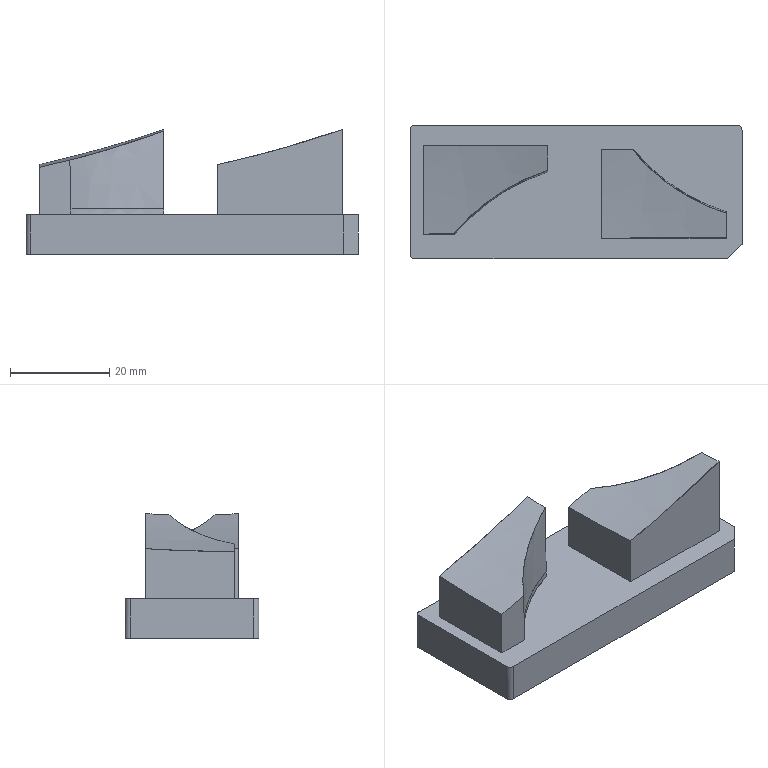NC program | PowerMill | posted with a generic post | part box 67 x 27 x 25.167 mm
Lines 1 to 966 of 102458:
%
O0001
N104 ( POWERMILL CB  : 2026004.0)
N105 ( POST VER      : 2026.0.0.5161)
N106 ( OPTION FILE   : FANUC)
N107 ( OUTPUT WORKPLANE : WORLD)
N108 (  )
N109 ( TOOL LIST )
N110 (---------------------------------------)
N111 ( NO. | ID        | DIA.| TIP RAD|LENGTH)
N112 (---------------------------------------)
N113 (    1|D10C_1_1_1 |10.0 |  0.0   | 80.6 )
N114 (    2|D4C_1_1    | 4.0 |  0.0   |72.36 )
N115 (    3|D10_1_1_1  |10.0 |  0.0   |80.32 )
N116 (    7|R2_1_1     | 4.0 |  2.0   |62.96 )
N117 (   14|D4_1_1     | 4.0 |  0.0   | 71.6 )
N118 (   13|TEXT_D4_1_1| 4.0 |  0.3   |72.44 )
N119 (---------------------------------------)
N120 (  )
N121 ( NUMBER OF TOOLPATHS: 11.0 )
N122 ( ESTIMATED PROGRAM DURATION: 0 HOURS 19 MIN 51 SEC)
N123 (  )
N124 G00 G21 G80 G40 G17
N125 G90
N126 G54
N127 G53 Z0.0
N128 (---------------)
N129 ( START TOOLPATH : 精公开粗01-扫面平行-D10C )
N130 (---------------)
N131 ( TOOL NO.    :1 )
N132 ( TOOL TYPE   : ENDMILL)
N133 ( TOOL ID     : D10C_1_1_1)
N134 ( TOOL DIA    : 10.0 LENGTH 80.6)
N135 T1
N136 M6
N137 S8000 M03
N138 G00 G90 X0.0 Y0.0
N139 G43 Z10.2 H1
N140
N141 G05 P10000 R4
N142 X41.28 Y16.28
N143 Z1.127
N144 G01 Z-0.073 F6000.0
N145 X36.28 F10000.0
N146 X-36.28
N147 Y10.8533
N148 X36.28
N149 Y5.4267
N150 X-36.28
N151 Y0.0
N152 X36.28
N153 Y-5.4267
N154 X-36.28
N155 Y-10.8533
N156 X36.28
N157 Y-16.28
N158 X-36.28
N159 X-41.28
N160 G00 Z10.2
N161 G05 P0
N162 (---------------)
N163 ( END TOOLPATH : 精公开粗01-扫面平行-D10C )
N164 (---------------)
N165 ( START TOOLPATH : 精公开粗01-外形偏置-D10C )
N166 (---------------)
N167 G00 X-0.268 Y0.0 Z9.877
N168 G05 P10000 R4
N169 X-11.5717 Y22.365
N170 Z0.6803
N171 G01 Z-0.5197 F6000.0
N172 Y21.8375 F10000.0
N173 G03 X-6.8242 Y17.09 I4.7475 J0.0
N174 G01 X37.09
N175 G02 X38.09 Y16.09 I0.0 J-1.0
N176 G01 Y-6.9606
N177 X35.5902 Y-6.9608
N178 X35.5904 Y-9.2811
N179 X35.5374 Y-10.0545
N180 X35.3673 Y-10.828
N181 X35.067 Y-11.6014
N182 X34.9229 Y-11.8793
N183 X34.6097 Y-12.3748
N184 X34.1495 Y-12.9347
N185 X33.9361 Y-13.1483
N186 X33.3761 Y-13.6088
N187 X32.8815 Y-13.9217
N188 X32.6026 Y-14.0665
N189 X31.8292 Y-14.3669
N190 X31.0558 Y-14.5372
N191 X30.2823 Y-14.5902
N192 X29.5089
N193 X28.7355 Y-14.5581
N194 X27.9621 Y-14.4258
N195 X27.1886 Y-14.1748
N196 X26.6483 Y-13.9217
N197 X26.4152 Y-13.7855
N198 X25.6418 Y-13.2108
N199 X24.885 Y-12.3748
N200 X24.4212 Y-11.6014
N201 X24.1176 Y-10.828
N202 X23.9457 Y-10.0545
N203 X23.892 Y-9.2811
N204 X23.9544 Y-8.5077
N205 X24.5442 Y-5.414
N206 X24.5451 Y-5.4084
N207 X24.9326 Y-3.0937
N208 X25.1686 Y-2.3203
N209 X25.5477 Y-1.5469
N210 X26.1094 Y-0.7734
N211 X26.4152 Y-0.4526
N212 X26.9613 Y0.0
N213 X27.1886 Y0.1604
N214 X27.9621 Y0.5754
N215 X28.7355 Y0.841
N216 X29.5089 Y0.9805
N217 X30.2823 Y1.0094
N218 X31.0558 Y0.9288
N219 X31.7201 Y0.7734
N220 X32.6026 Y0.4341
N221 X33.3761 Y-0.028
N222 X34.1495 Y-0.6979
N223 X34.7993 Y-1.5469
N224 X35.1956 Y-2.3203
N225 X35.4449 Y-3.0937
N226 X35.5703 Y-3.8671
N227 X35.59 Y-4.6406
N228 X35.5902 Y-6.9608
N229 X38.09 Y-6.9606
N230 Y-16.09
N231 G02 X37.09 Y-17.09 I-1.0 J0.0
N232 G01 X-22.2547
N233 X-22.5546 Y-11.206
N234 X-22.8367 Y-5.6714
N235 G03 X-21.277 Y-3.1512 I-0.0917 J1.7994
N236 G01 X-21.9484 Y-1.6131
N237 G02 X-23.1151 Y2.2109 I15.9046 J6.9426
N238 G01 X-23.4191 Y3.8745
N239 G03 X-25.1213 Y5.2492 I-1.6495 J-0.3013
N240 G01 X-25.5601 Y5.2354
N241 G03 X-27.1822 Y3.4765 I0.0527 J-1.676
N242 G01 X-26.8413 Y-3.4115
N243 G03 X-25.2109 Y-5.2787 I1.9975 J0.0988
N244 G01 X-23.2591 Y-5.6431
N245 X-23.0487 Y-5.6697
N246 X-22.8367 Y-5.6714
N247 X-22.5546 Y-11.206
N248 X-30.7368 Y-11.1992
N249 G02 X-32.7352 Y-9.1992 I0.0016 J2.0
N250 G01 Y9.1992
N251 G02 X-30.7496 Y11.1991 I2.0 J0.0
N252 G01 X-20.0092 Y11.2763
N253 G02 X-17.9956 Y9.3329 I0.0144 J-1.9999
N254 G01 X-17.8738 Y5.0263
N255 G03 X-4.3101 Y-6.4593 I11.9306 J0.3375
N256 G03 X5.6322 Y8.2731 I-1.6331 J11.8231
N257 G01 X5.5061 Y8.7748
N258 G02 X7.4513 Y11.2623 I1.9397 J0.4875
N259 G01 X30.2047 Y11.1992
N260 G02 X32.1103 Y9.7888 I-0.0055 J-2.0
N261 G01 X32.2036 Y9.4862
N262 G02 X30.5723 Y6.9163 I-1.9111 J-0.5896
N263 G01 X29.4818 Y6.7622
N264 G03 X18.7754 Y-2.4572 I1.8296 J-12.951
N265 G01 X13.4797 Y-0.8831
N266 G03 X12.8988 Y-3.5369 I17.7492 J-5.276
N267 G01 X12.8103 Y-4.1552
N268 G02 X10.533 Y-5.6329 I-1.7836 J0.2551
N269 G02 X9.3764 Y-3.1769 I0.4937 J1.7328
N270 G01 X10.0532 Y-1.6325
N271 G03 X11.0015 Y1.1532 I-15.8897 J6.9633
N272 G01 X11.7966 Y4.3577
N273 G02 X14.1246 Y5.6116 I1.7333 J-0.43
N274 G02 X15.1489 Y3.1738 I-0.5947 J-1.6839
N275 G01 X14.4427 Y1.6571
N276 G03 X13.4797 Y-0.8831 I16.7862 J-7.8162
N277 G01 X18.7754 Y-2.4572
N278 G03 X18.2448 Y-5.605 I12.5361 J-3.7317
N279 G01 X18.0785 Y-9.3272
N280 G02 X16.0788 Y-11.2379 I-1.998 J0.0893
N281 G01 X-22.5546 Y-11.206
N282 X-22.2547 Y-17.09
N283 X-37.626
N284 G02 X-38.626 Y-16.09 I0.0 J1.0
N285 G01 Y16.09
N286 G02 X-37.626 Y17.09 I1.0 J0.0
N287 G01 X-6.8242
N288 X-6.8421 Y14.5865
N289 X-5.2953 Y14.5754
N290 X-4.5218 Y14.4594
N291 X-3.7484 Y14.2202
N292 X-2.975 Y13.8387
N293 X-2.2016 Y13.2737
N294 X-2.0639 Y13.1483
N295 X-1.4281 Y12.4272
N296 X-0.9329 Y11.6014
N297 X-0.6547 Y10.8993
N298 X-0.4626 Y10.0545
N299 X-0.4096 Y9.2811
N300 X-0.4099 Y4.6406
N301 X-0.4415 Y3.8671
N302 X-0.559 Y3.0937
N303 X-0.6547 Y2.7306
N304 X-0.8078 Y2.3203
N305 X-1.2007 Y1.5469
N306 X-1.4281 Y1.2013
N307 X-1.7815 Y0.7734
N308 X-2.2016 Y0.3608
N309 X-2.6552 Y0.0
N310 X-2.975 Y-0.2075
N311 X-3.7484 Y-0.585
N312 X-4.28 Y-0.7734
N313 X-4.5218 Y-0.8397
N314 X-5.2953 Y-0.9791
N315 X-6.0687 Y-1.0112
N316 X-6.8421 Y-0.9328
N317 X-7.4993 Y-0.7734
N318 X-8.389 Y-0.4068
N319 X-9.0394 Y0.0
N320 X-9.891 Y0.7734
N321 X-10.4555 Y1.5469
N322 X-10.8319 Y2.3203
N323 X-11.0675 Y3.0937
N324 X-11.4557 Y5.414
N325 X-11.4567 Y5.4196
N326 X-12.0456 Y8.5077
N327 X-12.1078 Y9.2811
N328 X-12.0543 Y10.0545
N329 X-11.8823 Y10.828
N330 X-11.5788 Y11.6014
N331 X-11.115 Y12.3748
N332 X-10.7093 Y12.8669
N333 X-10.4304 Y13.1483
N334 X-9.9358 Y13.5525
N335 X-9.1624 Y14.0191
N336 X-8.389 Y14.3276
N337 X-7.6156 Y14.5118
N338 X-6.8421 Y14.5865
N339 X-6.8242 Y17.09
N340 G00 Z3.2837
N341 G01 X-11.5717 Y22.365
N342 G00 Z0.2837
N343 G01 Z-0.9163 F6000.0
N344 Y21.8375 F10000.0
N345 G03 X-6.8242 Y17.09 I4.7475 J0.0
N346 G01 X37.09
N347 G02 X38.09 Y16.09 I0.0 J-1.0
N348 G01 Y-6.9606
N349 X35.5902 Y-6.9608
N350 X35.5904 Y-9.2811
N351 X35.5374 Y-10.0545
N352 X35.3673 Y-10.828
N353 X35.0671 Y-11.6014
N354 X34.9229 Y-11.8793
N355 X34.6097 Y-12.3748
N356 X34.1495 Y-12.9347
N357 X33.9361 Y-13.1483
N358 X33.3761 Y-13.6088
N359 X32.8815 Y-13.9217
N360 X32.6026 Y-14.0665
N361 X31.8292 Y-14.3669
N362 X31.0558 Y-14.5372
N363 X30.2823 Y-14.5902
N364 X30.2489 Y-14.5901
N365 X29.5089
N366 X29.4801 Y-14.5889
N367 X27.9621 Y-14.5866
N368 X27.1886 Y-14.5132
N369 X26.4152 Y-14.3301
N370 X25.6418 Y-14.0219
N371 X25.443 Y-13.9217
N372 X24.8684 Y-13.5603
N373 X24.3646 Y-13.1483
N374 X24.0949 Y-12.8781
N375 X23.68 Y-12.3748
N376 X23.2159 Y-11.6014
N377 X22.9124 Y-10.828
N378 X22.7407 Y-10.0545
N379 X22.6864 Y-9.2811
N380 X22.7494 Y-8.5077
N381 X22.9123 Y-7.7343
N382 X23.3215 Y-5.5054
N383 X23.3221 Y-5.5019
N384 X23.7288 Y-3.0937
N385 X23.9005 Y-2.3203
N386 X24.2043 Y-1.5469
N387 X24.6723 Y-0.7734
N388 X24.8684 Y-0.523
N389 X25.3564 Y0.0
N390 X25.6418 Y0.2402
N391 X26.4152 Y0.753
N392 X27.1886 Y1.0949
N393 X27.9621 Y1.3019
N394 X28.7355 Y1.3898
N395 X29.5089 Y1.3668
N396 X30.2823 Y1.2353
N397 X31.8292 Y0.7479
N398 X32.6026 Y0.4454
N399 X33.3585 Y0.0
N400 X34.1495 Y-0.6863
N401 X34.8074 Y-1.5469
N402 X35.2005 Y-2.3203
N403 X35.4479 Y-3.0937
N404 X35.5714 Y-3.8671
N405 X35.59 Y-4.6406
N406 X35.5902 Y-6.9608
N407 X38.09 Y-6.9606
N408 Y-16.09
N409 G02 X37.09 Y-17.09 I-1.0 J0.0
N410 G01 X-37.626
N411 G02 X-38.626 Y-16.09 I0.0 J1.0
N412 G01 Y0.2381
N413 X-32.7352 Y0.2768
N414 X-27.0159 Y0.3143
N415 X-26.9911 Y-3.4731
N416 G03 X-25.074 Y-5.4583 I2.0 J0.0131
N417 G01 X-23.3985 Y-5.5278
N418 G03 X-22.2168 Y-3.728 I0.0521 J1.2536
N419 G01 X-22.7391 Y-2.6477
N420 G02 X-24.3628 Y2.8373 I15.9131 J7.6934
N421 G01 X-24.5433 Y4.271
N422 G03 X-25.7166 Y5.225 I-1.0857 J-0.1367
N423 G01 X-26.0341 Y5.1995
N424 G03 X-27.0407 Y4.1016 I0.0876 J-1.0907
N425 G01 X-27.0159 Y0.3143
N426 X-32.7352 Y0.2768
N427 Y9.1992
N428 G02 X-30.7514 Y11.1991 I2.0 J0.0
N429 G01 X-21.2163 Y11.2764
N430 G02 X-19.206 Y9.43 I0.0162 J-1.9999
N431 G01 X-18.7994 Y4.1489
N432 G03 X-11.2701 Y-6.1398 I12.0634 J0.9287
N433 G01 X-10.746 Y-6.3516
N434 G03 X5.7634 Y6.0495 I4.5174 J11.1759
N435 G01 X5.4559 Y9.059
N436 G02 X7.4511 Y11.2622 I1.9896 J0.2032
N437 G01 X30.2047 Y11.1992
N438 G02 X30.8927 Y11.0751 I-0.0055 J-2.0
N439 G01 X31.0608 Y11.0129
N440 G02 X30.3642 Y7.137 I-0.6935 J-1.8759
N441 G01 X29.8347 Y7.1378
N442 G03 X17.7003 Y-2.0045 I-0.0194 J-12.5982
N443 G01 X12.2512 Y-0.4246
N444 G03 X11.581 Y-3.9362 I18.367 J-5.3251
N445 G01 X11.5318 Y-4.4526
N446 G02 X10.0763 Y-5.4572 I-1.15 J0.1096
N447 G02 X9.3366 Y-3.8507 I0.3055 J1.1142
N448 G01 X9.5727 Y-3.3497
N449 G03 X11.4992 Y3.3019 I-19.8733 J9.3609
N450 G01 X11.6451 Y4.476
N451 G02 X13.2489 Y5.5161 I1.239 J-0.154
N452 G02 X13.9976 Y3.7572 I-0.3648 J-1.1941
N453 G01 X13.5633 Y2.9009
N454 G03 X12.2512 Y-0.4246 I17.055 J-8.6506
N455 G01 X17.7003 Y-2.0045
N456 G03 X17.2557 Y-4.4743 I12.115 J-3.4559
N457 G01 X16.8694 Y-9.3945
N458 G02 X14.8738 Y-11.2379 I-1.9939 J0.1566
N459 G01 X-30.7369 Y-11.1992
N460 G02 X-32.7352 Y-9.1992 I0.0017 J2.0
N461 G01 Y0.2768
N462 X-38.626 Y0.2381
N463 Y16.09
N464 G02 X-37.626 Y17.09 I1.0 J0.0
N465 G01 X-8.4669
N466 X-8.389 Y14.5662
N467 X-7.6156 Y14.5901
N468 X-6.8541 Y14.5853
N469 X-6.8421 Y14.5864
N470 X-5.3579 Y14.5758
N471 X-5.2953 Y14.5754
N472 X-4.5218 Y14.4594
N473 X-3.7484 Y14.2202
N474 X-2.975 Y13.8387
N475 X-2.2016 Y13.2737
N476 X-2.0639 Y13.1483
N477 X-1.4281 Y12.4272
N478 X-0.9329 Y11.6014
N479 X-0.6547 Y10.8993
N480 X-0.4626 Y10.0545
N481 X-0.4096 Y9.2811
N482 X-0.4099 Y4.6406
N483 X-0.4286 Y3.8671
N484 X-0.5521 Y3.0937
N485 X-0.6547 Y2.7222
N486 X-0.7995 Y2.3203
N487 X-1.1925 Y1.5469
N488 X-1.4281 Y1.1939
N489 X-1.7717 Y0.7734
N490 X-2.2016 Y0.3474
N491 X-2.6414 Y0.0
N492 X-2.975 Y-0.2173
N493 X-3.7484 Y-0.5992
N494 X-4.2475 Y-0.7734
N495 X-5.2953 Y-1.1191
N496 X-6.0687 Y-1.3091
N497 X-6.8421 Y-1.3915
N498 X-7.6156 Y-1.3642
N499 X-8.389 Y-1.2241
N500 X-9.1624 Y-0.9594
N501 X-9.5528 Y-0.7734
N502 X-9.9358 Y-0.5445
N503 X-10.6395 Y0.0
N504 X-11.3283 Y0.7734
N505 X-11.7969 Y1.5469
N506 X-12.0994 Y2.3203
N507 X-12.2561 Y3.0081
N508 X-12.8026 Y6.1874
N509 X-12.8036 Y6.1925
N510 X-13.2507 Y8.5077
N511 X-13.3131 Y9.2811
N512 X-13.2593 Y10.0545
N513 X-13.0873 Y10.828
N514 X-12.7842 Y11.6014
N515 X-12.32 Y12.3748
N516 X-11.6354 Y13.1483
N517 X-11.4827 Y13.2813
N518 X-10.7093 Y13.8341
N519 X-9.9358 Y14.2081
N520 X-9.1624 Y14.4445
N521 X-8.389 Y14.5662
N522 X-8.4669 Y17.09
N523 X-6.8242
N524 G00 Z2.887
N525 G01 X-11.5717 Y22.365
N526 G00 Z-0.113
N527 G01 Z-1.313 F6000.0
N528 Y21.8375 F10000.0
N529 G03 X-6.8242 Y17.09 I4.7475 J0.0
N530 G01 X37.09
N531 G02 X38.09 Y16.09 I0.0 J-1.0
N532 G01 Y-6.9606
N533 X35.5902 Y-6.9608
N534 X35.5904 Y-9.2811
N535 X35.5374 Y-10.0545
N536 X35.3673 Y-10.828
N537 X35.0671 Y-11.6014
N538 X34.9229 Y-11.8793
N539 X34.6097 Y-12.3748
N540 X34.1495 Y-12.9347
N541 X33.9361 Y-13.1483
N542 X33.3761 Y-13.6088
N543 X32.8815 Y-13.9217
N544 X32.6026 Y-14.0665
N545 X31.8292 Y-14.3669
N546 X31.0558 Y-14.5372
N547 X30.2823 Y-14.5902
N548 X27.1886
N549 X26.4152 Y-14.5672
N550 X25.6418 Y-14.4464
N551 X24.8684 Y-14.2116
N552 X24.2377 Y-13.9217
N553 X23.3215 Y-13.2891
N554 X23.1596 Y-13.1483
N555 X22.5481 Y-12.4699
N556 X22.0106 Y-11.6014
N557 X21.7072 Y-10.828
N558 X21.5357 Y-10.0545
N559 X21.4809 Y-9.2811
N560 X21.5444 Y-8.5077
N561 X21.7037 Y-7.7343
N562 X21.7047 Y-7.7287
N563 X22.2687 Y-4.6406
N564 X22.6453 Y-2.3203
N565 X22.872 Y-1.5469
N566 X23.2412 Y-0.7734
N567 X23.7936 Y0.0
N568 X24.0949 Y0.3188
N569 X24.6231 Y0.7734
N570 X24.8684 Y0.9443
N571 X25.6418 Y1.3697
N572 X26.0916 Y1.5469
N573 X26.4152 Y1.6445
N574 X27.1886 Y1.7907
N575 X27.9621 Y1.8247
N576 X28.7355 Y1.7476
N577 X29.5089 Y1.5615
N578 X31.8292 Y0.7551
N579 X32.6026 Y0.4526
N580 X33.3685 Y0.0
N581 X34.1495 Y-0.6791
N582 X34.8133 Y-1.5469
N583 X35.2034 Y-2.3203
N584 X35.4496 Y-3.0937
N585 X35.5721 Y-3.8671
N586 X35.59 Y-4.6406
N587 X35.5902 Y-6.9608
N588 X38.09 Y-6.9606
N589 Y-16.09
N590 G02 X37.09 Y-17.09 I-1.0 J0.0
N591 G01 X-37.626
N592 G02 X-38.626 Y-16.09 I0.0 J1.0
N593 G01 Y-1.2302
N594 X-32.7352 Y-1.1964
N595 X-27.19 Y-1.1646
N596 X-27.1748 Y-3.8177
N597 G03 X-24.9559 Y-5.6381 I1.865 J0.0107
N598 G03 X-23.5752 Y-3.122 I-0.3539 J1.8311
N599 G01 X-24.2046 Y-1.5282
N600 G02 X-24.9112 Y0.6505 I17.06 J6.7369
N601 G01 X-25.1929 Y1.7485
N602 G03 X-27.2052 Y1.4886 I-0.9901 J-0.254
N603 G01 X-27.19 Y-1.1646
N604 X-32.7352 Y-1.1964
N605 Y9.1992
N606 G02 X-30.7538 Y11.1991 I2.0 J0.0
N607 G01 X-22.4239 Y11.2766
N608 G02 X-20.4138 Y9.4606 I0.0186 J-2.0
N609 G01 X-19.9158 Y4.0679
N610 G03 X-4.8861 Y-7.5416 I12.9204 J1.1932
N611 G03 X5.9641 Y4.6207 I-2.1093 J12.8027
N612 G01 X11.6498
N613 G02 X13.073 I0.7116 J0.0
N614 G02 X11.6498 I-0.7116 J0.0
N615 G01 X5.9641
N616 G03 X5.6248 Y8.2759 I-12.9595 J0.6404
N617 G01 X5.5002 Y8.7975
N618 G02 X7.4402 Y11.2622 I1.9453 J0.4647
N619 G01 X30.439 Y11.3237
N620 G02 X32.4412 Y9.2119 I0.0053 J-2.0
N621 G02 X30.2159 Y7.3368 I-1.9969 J0.1118
N622 G01 X29.7019 Y7.3959
N623 G03 X16.5023 Y-2.9308 I-1.3634 J-11.8566
N624 G01 X15.654 Y-9.4943
N625 G02 X13.6687 Y-11.2379 I-1.9835 J0.2564
N626 G01 X9.679 Y-11.2344
N627 Y-5.0582
N628 G02 X9.4663 Y-4.8455 I0.0 J0.2127
N629 G02 X9.8917 I0.2127 J0.0
N630 G02 X9.679 Y-5.0582 I-0.2127 J0.0
N631 G01 Y-11.2344
N632 X-30.7369 Y-11.1992
N633 G02 X-32.7352 Y-9.1992 I0.0017 J2.0
N634 G01 Y-1.1964
N635 X-38.626 Y-1.2302
N636 Y16.09
N637 G02 X-37.626 Y17.09 I1.0 J0.0
N638 G01 X-9.1535
N639 X-9.1624 Y14.5891
N640 X-7.8012 Y14.5843
N641 X-7.6156 Y14.59
N642 X-6.8541 Y14.5852
N643 X-6.8421 Y14.5864
N644 X-5.3579 Y14.5757
N645 X-5.314 Y14.5755
N646 X-5.2953 Y14.5754
N647 X-4.5218 Y14.4594
N648 X-3.7484 Y14.2202
N649 X-2.975 Y13.8387
N650 X-2.2016 Y13.2737
N651 X-2.0639 Y13.1483
N652 X-1.4281 Y12.4272
N653 X-0.9329 Y11.6014
N654 X-0.6547 Y10.8993
N655 X-0.4626 Y10.0545
N656 X-0.4096 Y9.2811
N657 X-0.407 Y8.5077
N658 X-0.4097 Y7.9099
N659 X-0.41 Y4.6406
N660 X-0.4278 Y3.9007
N661 X-0.4279 Y3.8671
N662 X-0.5504 Y3.0937
N663 X-0.6547 Y2.7145
N664 X-0.7966 Y2.3203
N665 X-1.1867 Y1.5469
N666 X-1.4281 Y1.1866
N667 X-1.7636 Y0.7734
N668 X-2.2016 Y0.3401
N669 X-2.6315 Y0.0
N670 X-2.975 Y-0.2249
N671 X-3.7484 Y-0.6064
N672 X-5.2953 Y-1.1279
N673 X-5.3011 Y-1.13
N674 X-6.443 Y-1.5469
N675 X-6.8421 Y-1.6601
N676 X-7.6156 Y-1.7967
N677 X-8.389 Y-1.8227
N678 X-9.1624 Y-1.7411
N679 X-9.9107 Y-1.5469
N680 X-10.7093 Y-1.2017
N681 X-11.3744 Y-0.7734
N682 X-12.2063 Y0.0
N683 X-12.7592 Y0.7734
N684 X-13.1274 Y1.5469
N685 X-13.3551 Y2.3203
N686 X-13.7306 Y4.6406
N687 X-14.4557 Y8.5077
N688 X-14.5184 Y9.2811
N689 X-14.4643 Y10.0545
N690 X-14.2923 Y10.828
N691 X-13.9895 Y11.6014
N692 X-13.803 Y11.9425
N693 X-13.525 Y12.3748
N694 X-13.0295 Y12.9591
N695 X-12.8404 Y13.1483
N696 X-12.2561 Y13.6173
N697 X-11.7615 Y13.9217
N698 X-11.4827 Y14.0613
N699 X-10.7093 Y14.3548
N700 X-9.9358 Y14.5249
N701 X-9.1624 Y14.5891
N702 X-9.1535 Y17.09
N703 X-6.8242
N704 G00 Z2.4903
N705 G01 X-11.5717 Y22.365
N706 G00 Z-0.5097
N707 G01 Z-1.7097 F6000.0
N708 Y21.8375 F10000.0
N709 G03 X-6.8242 Y17.09 I4.7475 J0.0
N710 G01 X37.09
N711 G02 X38.09 Y16.09 I0.0 J-1.0
N712 G01 Y-6.9528
N713 X35.5902 Y-6.953
N714 X35.5904 Y-9.2655
N715 Y-9.2811
N716 X35.5374 Y-10.0545
N717 X35.3673 Y-10.828
N718 X35.0671 Y-11.6014
N719 X34.9229 Y-11.8793
N720 X34.6097 Y-12.3748
N721 X34.1495 Y-12.9347
N722 X33.9361 Y-13.1483
N723 X33.3761 Y-13.6088
N724 X32.8815 Y-13.9217
N725 X32.6026 Y-14.0665
N726 X31.8292 Y-14.3669
N727 X31.0558 Y-14.5373
N728 X30.2823 Y-14.5902
N729 X29.9557 Y-14.5901
N730 X27.1886
N731 X27.1735 Y-14.5897
N732 X25.6418 Y-14.5894
N733 X24.8684 Y-14.5311
N734 X24.0949 Y-14.369
N735 X23.3215 Y-14.0833
N736 X22.9931 Y-13.9217
N737 X22.5481 Y-13.6501
N738 X21.9106 Y-13.1483
N739 X21.2247 Y-12.3748
N740 X20.7642 Y-11.6014
N741 X20.4603 Y-10.828
N742 X20.2876 Y-10.0545
N743 X20.2354 Y-9.2811
N744 X20.2956 Y-8.5077
N745 X20.4643 Y-7.7343
N746 X21.0458 Y-4.6406
N747 X21.3943 Y-2.3203
N748 X21.5539 Y-1.5469
N749 X21.7747 Y-0.9121
N750 X22.2665 Y0.0
N751 X22.5481 Y0.3753
N752 X22.9064 Y0.7734
N753 X23.3215 Y1.145
N754 X23.8934 Y1.5469
N755 X24.0949 Y1.6624
N756 X24.8684 Y2.004
N757 X25.6418 Y2.213
N758 X26.4152 Y2.2992
N759 X27.1886 Y2.2755
N760 X27.9621 Y2.1415
N761 X28.7355 Y1.8957
N762 X30.1515 Y1.3381
N763 X30.983 Y1.0491
N764 X31.8292 Y0.7624
N765 X32.6026 Y0.4599
N766 X33.3784 Y0.0
N767 X34.1495 Y-0.6718
N768 X34.8177 Y-1.5469
N769 X35.2064 Y-2.3203
N770 X35.4513 Y-3.0937
N771 X35.5727 Y-3.8671
N772 X35.5728 Y-3.8996
N773 X35.59 Y-4.6406
N774 X35.5902 Y-6.953
N775 X38.09 Y-6.9528
N776 Y-16.09
N777 G02 X37.09 Y-17.09 I-1.0 J0.0
N778 G01 X-37.626
N779 G02 X-38.626 Y-16.09 I0.0 J1.0
N780 G01 Y0.0176
N781 X-32.7352
N782 X-27.2382
N783 Y-5.6846
N784 X-27.2321 Y-5.6993
N785 X-27.2174 Y-5.7054
N786 X-23.3652 Y-5.7088
N787 X-23.3551 Y-5.7028
N788 X-23.3557 Y-5.691
N789 X-23.3864 Y-5.6463
N790 G02 X-26.5536 Y3.0502 I15.3812 J10.5269
N791 G01 X-26.8175 Y5.7241
N792 X-26.8251 Y5.7391
N793 X-26.8408 Y5.745
N794 X-27.2174 Y5.7408
N795 X-27.2321 Y5.7346
N796 X-27.2382 Y5.7198
N797 Y0.0176
N798 X-32.7352
N799 Y9.1992
N800 G02 X-30.7573 Y11.1991 I2.0 J0.0
N801 G01 X-23.6762 Y11.2773
N802 G02 X-21.6637 Y9.4737 I0.0221 J-1.9999
N803 G01 X-21.0834 Y3.5907
N804 G03 X3.4691 Y-1.5292 I13.0791 J1.2902
N805 G01 X3.9917 Y-0.5937
N806 G03 X5.262 Y2.5185 I-12.0578 J6.7366
N807 G01 X10.5663 Y1.076
N808 G03 X11.2385 Y5.7271 I-18.6324 J5.0669
N809 G01 X11.2395 Y5.776
N810 X11.2459 Y5.7908
N811 X11.2608 Y5.797
N812 X12.7863 Y5.8098
N813 X12.7965 Y5.8038
N814 X12.7959 Y5.7921
N815 X12.7703 Y5.7537
N816 G03 X10.0686 Y-1.2589 I14.2778 J-9.5275
N817 G01 X9.4083 Y-5.7171
N818 X9.3999 Y-5.7323
N819 X9.3835 Y-5.7384
N820 X7.3375 Y-5.7366
N821 X7.3274 Y-5.7305
N822 X7.3281 Y-5.7187
N823 X7.3553 Y-5.6791
N824 X7.8284 Y-4.9556
N825 X8.2675 Y-4.2109
N826 X8.7904 Y-3.2749
N827 G03 X10.5663 Y1.076 I-16.8565 J9.4178
N828 G01 X5.262 Y2.5185
N829 G03 X5.5616 Y8.3925 I-13.3281 J3.6244
N830 G01 X5.4718 Y8.9362
N831 G02 X7.4283 Y11.2619 I1.9733 J0.3258
N832 G01 X30.5028 Y11.4561
N833 G02 X32.5085 Y9.2459 I0.0168 J-1.9999
N834 G02 X30.0849 Y7.504 I-1.9889 J0.2103
N835 G01 X29.5848 Y7.6154
N836 G03 X15.5061 Y-2.0646 I-2.5362 J-11.3894
N837 G01 X14.4004 Y-9.5311
N838 G02 X12.4202 Y-11.2381 I-1.9784 J0.293
N839 G01 X-30.737 Y-11.1992
N840 G02 X-32.7352 Y-9.1992 I0.0018 J2.0
N841 G01 Y0.0176
N842 X-38.626
N843 Y16.09
N844 G02 X-37.626 Y17.09 I1.0 J0.0
N845 G01 X-10.7091
N846 X-10.7093 Y14.5757
N847 X-9.3251 Y14.5756
N848 X-9.1624 Y14.5891
N849 X-7.8012 Y14.5843
N850 X-7.6156 Y14.59
N851 X-6.8541 Y14.5852
N852 X-6.8421 Y14.5863
N853 X-5.3579 Y14.5757
N854 X-5.314 Y14.5754
N855 X-5.3103
N856 X-5.2953
N857 X-4.5218 Y14.4594
N858 X-3.7484 Y14.2202
N859 X-2.975 Y13.8387
N860 X-2.2016 Y13.2737
N861 X-2.0639 Y13.1483
N862 X-1.4281 Y12.4272
N863 X-0.9329 Y11.6014
N864 X-0.6547 Y10.8993
N865 X-0.4626 Y10.0545
N866 X-0.4096 Y9.2811
N867 Y9.2732
N868 X-0.4071 Y8.5077
N869 X-0.4098 Y7.9099
N870 X-0.41 Y4.6406
N871 X-0.4271 Y3.9297
N872 X-0.4273 Y3.8671
N873 X-0.5487 Y3.0937
N874 X-0.6547 Y2.7072
N875 X-0.7936 Y2.3203
N876 X-1.1823 Y1.5469
N877 X-1.4281 Y1.1794
N878 X-1.7571 Y0.7734
N879 X-2.2016 Y0.3328
N880 X-2.6215 Y0.0
N881 X-2.975 Y-0.2321
N882 X-3.7484 Y-0.6137
N883 X-5.2953 Y-1.1351
N884 X-6.41 Y-1.5469
N885 X-6.415 Y-1.5488
N886 X-7.6156 Y-2.0222
N887 X-8.389 Y-2.2168
N888 X-9.1624 Y-2.3
N889 X-9.9358 Y-2.2742
N890 X-10.7093 Y-2.1327
N891 X-11.4827 Y-1.8688
N892 X-12.1059 Y-1.5469
N893 X-13.0295 Y-0.8353
N894 X-13.7331 Y0.0
N895 X-14.1665 Y0.7734
N896 X-14.4465 Y1.5469
N897 X-14.5764 Y2.144
N898 X-14.8367 Y3.8671
N899 X-15.3498 Y6.8109
N900 X-15.7036 Y8.5077
N901 X-15.7677 Y9.2811
N902 X-15.7117 Y10.0545
N903 X-15.5413 Y10.828
N904 X-15.2369 Y11.6014
N905 X-14.7735 Y12.3748
N906 X-14.5764 Y12.6262
N907 X-14.0882 Y13.1483
N908 X-13.803 Y13.3925
N909 X-13.0091 Y13.9217
N910 X-12.2561 Y14.2565
N911 X-11.4827 Y14.4708
N912 X-10.7093 Y14.5757
N913 X-10.7091 Y17.09
N914 X-6.8242
N915 G00 Z2.0936
N916 G01 X-11.5717 Y22.365
N917 G00 Z-0.9064
N918 G01 Z-2.1064 F6000.0
N919 Y21.8375 F10000.0
N920 G03 X-6.8242 Y17.09 I4.7475 J0.0
N921 G01 X37.09
N922 G02 X38.09 Y16.09 I0.0 J-1.0
N923 G01 Y-6.9439
N924 X35.5901 Y-6.9441
N925 X35.5903 Y-9.2476
N926 X35.5904 Y-9.2811
N927 X35.5374 Y-10.0545
N928 X35.3673 Y-10.828
N929 X35.0671 Y-11.6014
N930 X34.9229 Y-11.8793
N931 X34.6097 Y-12.3748
N932 X34.1495 Y-12.9347
N933 X33.9361 Y-13.1483
N934 X33.3761 Y-13.6088
N935 X32.8815 Y-13.9217
N936 X32.6026 Y-14.0665
N937 X31.8292 Y-14.3669
N938 X31.0558 Y-14.5373
N939 X30.2823 Y-14.5902
N940 X30.2431 Y-14.5901
N941 X29.9557
N942 X27.1886
N943 X27.1735 Y-14.5896
N944 X25.6418 Y-14.5894
N945 X25.5594 Y-14.5832
N946 X24.0949 Y-14.581
N947 X23.3215 Y-14.4883
N948 X22.5481 Y-14.2851
N949 X21.7747 Y-13.9532
N950 X21.0012 Y-13.4556
N951 X20.6307 Y-13.1483
N952 X20.2278 Y-12.726
N953 X19.9436 Y-12.3748
N954 X19.4836 Y-11.6014
N955 X19.1798 Y-10.828
N956 X19.0073 Y-10.0545
N957 X18.9548 Y-9.2811
N958 X19.0156 Y-8.5077
N959 X19.1931 Y-7.7343
N960 X19.7656 Y-4.6406
N961 X20.2278 Y-1.692
N962 X20.449 Y-0.7734
N963 X20.7741 Y0.0
N964 X21.0012 Y0.4014
N965 X21.2613 Y0.7734
N966 X21.7747 Y1.3498
N967 X21.9904 Y1.5469
N968 X22.5481 Y1.9695
N969 X23.1692 Y2.3203
N970 X24.0949 Y2.6569
N971 X24.8684 Y2.7987
N972 X25.6418 Y2.8274
N973 X26.4152 Y2.7455
N974 X27.1886 Y2.5498
N975 X27.7857 Y2.3203
N976 X28.7355 Y1.9032
N977 X30.2823 Y1.2948
N978 X30.2936 Y1.291
N979 X31.8292 Y0.7696
N980 X32.6026 Y0.4672
N981 X33.3761 Y0.0095
N982 X34.1495 Y-0.6646
N983 X34.8221 Y-1.5469
N984 X35.2093 Y-2.3203
N985 X35.453 Y-3.0937
N986 X35.5732 Y-3.8671
N987 X35.5734 Y-3.9311
N988 X35.59 Y-4.6406
N989 X35.5901 Y-6.9441
N990 X38.09 Y-6.9439
N991 Y-16.09
N992 G02 X37.09 Y-17.09 I-1.0 J0.0
N993 G01 X-37.626
N994 G02 X-38.626 Y-16.09 I0.0 J1.0
N995 G01 Y16.09
N996 G02 X-37.626 Y17.09 I1.0 J0.0
N997 G01 X-11.8039
N998 X-11.676 Y14.5803
N999 X-11.4827 Y14.5901
N1000 X-9.2144 Y14.5847
N1001 X-9.1624 Y14.589
N1002 X-7.8012 Y14.5842
N1003 X-7.6155 Y14.5899
N1004 X-6.8541 Y14.5851
N1005 X-6.8421 Y14.5863
N1006 X-5.3579 Y14.5756
N1007 X-5.3336 Y14.5755
N1008 X-5.2953 Y14.5754
N1009 X-4.5218 Y14.4594
N1010 X-3.7484 Y14.2202
N1011 X-2.975 Y13.8387
N1012 X-2.2016 Y13.2737
N1013 X-2.0639 Y13.1483
N1014 X-1.4281 Y12.4272
N1015 X-0.9329 Y11.6014
N1016 X-0.6547 Y10.8994
N1017 X-0.4626 Y10.0545
N1018 X-0.4096 Y9.2811
N1019 Y9.2651
N1020 X-0.4071 Y8.5077
N1021 X-0.4098 Y7.9099
N1022 X-0.4101 Y4.6406
N1023 X-0.4265 Y3.9599
N1024 X-0.4268 Y3.8671
N1025 X-0.547 Y3.0937
N1026 X-0.6547 Y2.7
N1027 X-0.7907 Y2.3203
N1028 X-1.1779 Y1.5469
N1029 X-1.4281 Y1.1721
N1030 X-1.7506 Y0.7734
N1031 X-2.2016 Y0.3256
N1032 X-2.6116 Y0.0
N1033 X-2.975 Y-0.2394
N1034 X-3.7484 Y-0.6209
N1035 X-5.2953 Y-1.1428
N1036 X-6.8421 Y-1.7289
N1037 X-8.2148 Y-2.3203
N1038 X-9.1624 Y-2.653
N1039 X-9.9358 Y-2.7974
N1040 X-10.7093 Y-2.83
N1041 X-11.4827 Y-2.7509
N1042 X-12.2561 Y-2.5539
N1043 X-13.0295 Y-2.2202
N1044 X-13.803 Y-1.7186
N1045 X-14.0099 Y-1.5469
N1046 X-14.5764 Y-0.9742
N1047 X-14.7399 Y-0.7734
N1048 X-15.2271 Y0.0
N1049 X-15.5511 Y0.7734
N1050 X-15.5609 Y0.8138
N1051 X-20.9434 Y-1.8015
N1052 X-25.1002 Y-3.8213
N1053 X-25.4087 Y-3.1864
N1054 X-25.7209 Y-2.5083
N1055 X-26.0045 Y-1.8178
N1056 X-26.3615 Y-0.8943
N1057 G03 X-28.1237 Y-1.2967 I-0.8518 J-0.3293
N1058 G01 X-27.8512 Y-4.6935
N1059 G03 X-27.6747 Y-5.3347 I1.7678 J0.1418
N1060 G01 X-27.464 Y-5.7629
N1061 G03 X-24.7917 Y-4.4562 I1.3345 J0.6566
N1062 G01 X-25.1002 Y-3.8213
N1063 X-20.9434 Y-1.8015